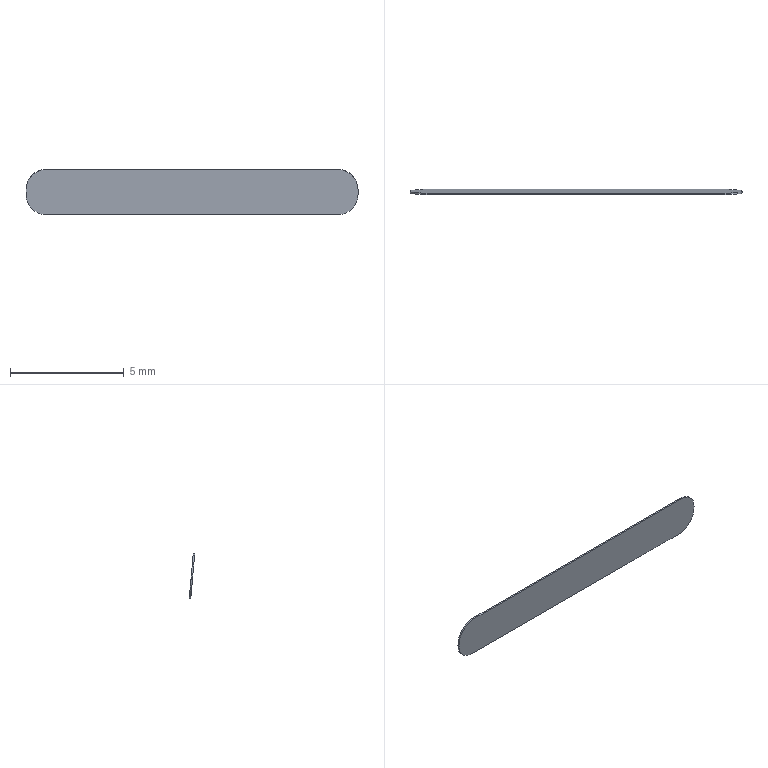Part | STEP file | p9-frame-03 | 1 solid | 10 faces | box 14.62 x 0.2371 x 1.998 mm | volume 1.798 mm3 | plane 6 | cylinder 4 | commonest cylinder face diameters 1.8 x4
STEP:
#1=CARTESIAN_POINT('',(27.35,-75.24,0.03301));
#2=VERTEX_POINT('',#1);
#3=CARTESIAN_POINT('',(26.45,-75.318,0.9296));
#4=VERTEX_POINT('',#3);
#5=CARTESIAN_POINT('',(26.45,-75.24,0.03301));
#6=DIRECTION('',(0.,-0.9962,-0.08716));
#7=DIRECTION('',(0.,-0.08716,0.9962));
#8=AXIS2_PLACEMENT_3D('',#5,#6,#7);
#9=CIRCLE('',#8,0.9);
#10=EDGE_CURVE('',#2,#4,#9,.T.);
#11=ORIENTED_EDGE('',*,*,#10,.F.);
#12=CARTESIAN_POINT('',(27.35,-75.222,-0.1662));
#13=VERTEX_POINT('',#12);
#14=CARTESIAN_POINT('',(27.35,-75.294,0.6557));
#15=DIRECTION('',(0.,-0.08716,0.9962));
#16=VECTOR('',#15,1000.);
#17=LINE('',#14,#16);
#18=EDGE_CURVE('',#13,#2,#17,.T.);
#19=ORIENTED_EDGE('',*,*,#18,.F.);
#20=CARTESIAN_POINT('',(26.45,-75.144,-1.063));
#21=VERTEX_POINT('',#20);
#22=CARTESIAN_POINT('',(26.45,-75.222,-0.1662));
#23=DIRECTION('',(0.,-0.9962,-0.08716));
#24=DIRECTION('',(0.,-0.08716,0.9962));
#25=AXIS2_PLACEMENT_3D('',#22,#23,#24);
#26=CIRCLE('',#25,0.9);
#27=EDGE_CURVE('',#21,#13,#26,.T.);
#28=ORIENTED_EDGE('',*,*,#27,.F.);
#29=CARTESIAN_POINT('',(13.63,-75.144,-1.063));
#30=VERTEX_POINT('',#29);
#31=CARTESIAN_POINT('',(2.234,-75.144,-1.063));
#32=DIRECTION('',(1.,0.,0.));
#33=VECTOR('',#32,1000.);
#34=LINE('',#31,#33);
#35=EDGE_CURVE('',#30,#21,#34,.T.);
#36=ORIENTED_EDGE('',*,*,#35,.F.);
#37=CARTESIAN_POINT('',(12.73,-75.222,-0.1662));
#38=VERTEX_POINT('',#37);
#39=CARTESIAN_POINT('',(13.63,-75.222,-0.1662));
#40=DIRECTION('',(0.,-0.9962,-0.08716));
#41=DIRECTION('',(0.,-0.08716,0.9962));
#42=AXIS2_PLACEMENT_3D('',#39,#40,#41);
#43=CIRCLE('',#42,0.9);
#44=EDGE_CURVE('',#38,#30,#43,.T.);
#45=ORIENTED_EDGE('',*,*,#44,.F.);
#46=CARTESIAN_POINT('',(12.73,-75.24,0.03301));
#47=VERTEX_POINT('',#46);
#48=CARTESIAN_POINT('',(12.73,-75.294,0.6557));
#49=DIRECTION('',(0.,0.08716,-0.9962));
#50=VECTOR('',#49,1000.);
#51=LINE('',#48,#50);
#52=EDGE_CURVE('',#47,#38,#51,.T.);
#53=ORIENTED_EDGE('',*,*,#52,.F.);
#54=CARTESIAN_POINT('',(13.63,-75.318,0.9296));
#55=VERTEX_POINT('',#54);
#56=CARTESIAN_POINT('',(13.63,-75.24,0.03301));
#57=DIRECTION('',(0.,-0.9962,-0.08716));
#58=DIRECTION('',(0.,-0.08716,0.9962));
#59=AXIS2_PLACEMENT_3D('',#56,#57,#58);
#60=CIRCLE('',#59,0.9);
#61=EDGE_CURVE('',#55,#47,#60,.T.);
#62=ORIENTED_EDGE('',*,*,#61,.F.);
#63=CARTESIAN_POINT('',(2.234,-75.318,0.9296));
#64=DIRECTION('',(-1.,0.,0.));
#65=VECTOR('',#64,1000.);
#66=LINE('',#63,#65);
#67=EDGE_CURVE('',#4,#55,#66,.T.);
#68=ORIENTED_EDGE('',*,*,#67,.F.);
#69=EDGE_LOOP('',(#11,#19,#28,#36,#45,#53,#62,#68));
#70=FACE_OUTER_BOUND('',#69,.T.);
#71=CARTESIAN_POINT('',(2.234,-75.294,0.6557));
#72=DIRECTION('',(0.,-0.9962,-0.08716));
#73=DIRECTION('',(0.,0.08716,-0.9962));
#74=AXIS2_PLACEMENT_3D('',#71,#72,#73);
#75=PLANE('',#74);
#76=ADVANCED_FACE('',(#70),#75,.F.);
#77=CARTESIAN_POINT('',(26.45,-75.381,0.9241));
#78=VERTEX_POINT('',#77);
#79=CARTESIAN_POINT('',(26.45,-75.717,0.8947));
#80=DIRECTION('',(0.,-0.9962,-0.08716));
#81=VECTOR('',#80,1000.);
#82=LINE('',#79,#81);
#83=EDGE_CURVE('',#4,#78,#82,.T.);
#84=ORIENTED_EDGE('',*,*,#83,.F.);
#85=ORIENTED_EDGE('',*,*,#67,.T.);
#86=CARTESIAN_POINT('',(13.63,-75.381,0.9241));
#87=VERTEX_POINT('',#86);
#88=CARTESIAN_POINT('',(13.63,-75.717,0.8947));
#89=DIRECTION('',(0.,0.9962,0.08716));
#90=VECTOR('',#89,1000.);
#91=LINE('',#88,#90);
#92=EDGE_CURVE('',#87,#55,#91,.T.);
#93=ORIENTED_EDGE('',*,*,#92,.F.);
#94=CARTESIAN_POINT('',(-31.59,-75.381,0.9241));
#95=DIRECTION('',(-1.,0.,0.));
#96=VECTOR('',#95,1000.);
#97=LINE('',#94,#96);
#98=EDGE_CURVE('',#78,#87,#97,.T.);
#99=ORIENTED_EDGE('',*,*,#98,.F.);
#100=EDGE_LOOP('',(#84,#85,#93,#99));
#101=FACE_OUTER_BOUND('',#100,.T.);
#102=CARTESIAN_POINT('',(-31.59,-75.717,0.8947));
#103=DIRECTION('',(0.,0.08716,-0.9962));
#104=DIRECTION('',(0.,0.9962,0.08716));
#105=AXIS2_PLACEMENT_3D('',#102,#103,#104);
#106=PLANE('',#105);
#107=ADVANCED_FACE('',(#101),#106,.F.);
#108=CARTESIAN_POINT('',(27.35,-75.302,0.02752));
#109=VERTEX_POINT('',#108);
#110=CARTESIAN_POINT('',(27.35,-76.511,-0.07823));
#111=DIRECTION('',(0.,0.9962,0.08716));
#112=VECTOR('',#111,1000.);
#113=LINE('',#110,#112);
#114=EDGE_CURVE('',#109,#2,#113,.T.);
#115=ORIENTED_EDGE('',*,*,#114,.T.);
#116=ORIENTED_EDGE('',*,*,#10,.T.);
#117=ORIENTED_EDGE('',*,*,#83,.T.);
#118=CARTESIAN_POINT('',(26.45,-75.302,0.02752));
#119=DIRECTION('',(0.,0.9962,0.08716));
#120=DIRECTION('',(0.,-0.08716,0.9962));
#121=AXIS2_PLACEMENT_3D('',#118,#119,#120);
#122=CIRCLE('',#121,0.9);
#123=EDGE_CURVE('',#78,#109,#122,.T.);
#124=ORIENTED_EDGE('',*,*,#123,.T.);
#125=EDGE_LOOP('',(#115,#116,#117,#124));
#126=FACE_OUTER_BOUND('',#125,.T.);
#127=CARTESIAN_POINT('',(26.45,-76.511,-0.07823));
#128=DIRECTION('',(0.,0.9962,0.08716));
#129=DIRECTION('',(0.,-0.08716,0.9962));
#130=AXIS2_PLACEMENT_3D('',#127,#128,#129);
#131=CYLINDRICAL_SURFACE('',#130,0.9);
#132=ADVANCED_FACE('',(#126),#131,.T.);
#133=ORIENTED_EDGE('',*,*,#18,.T.);
#134=ORIENTED_EDGE('',*,*,#114,.F.);
#135=CARTESIAN_POINT('',(27.35,-75.285,-0.1717));
#136=VERTEX_POINT('',#135);
#137=CARTESIAN_POINT('',(27.35,-75.302,0.02752));
#138=DIRECTION('',(0.,0.08716,-0.9962));
#139=VECTOR('',#138,1000.);
#140=LINE('',#137,#139);
#141=EDGE_CURVE('',#109,#136,#140,.T.);
#142=ORIENTED_EDGE('',*,*,#141,.T.);
#143=CARTESIAN_POINT('',(27.35,-75.285,-0.1717));
#144=DIRECTION('',(0.,0.9962,0.08716));
#145=VECTOR('',#144,1000.);
#146=LINE('',#143,#145);
#147=EDGE_CURVE('',#136,#13,#146,.T.);
#148=ORIENTED_EDGE('',*,*,#147,.T.);
#149=EDGE_LOOP('',(#133,#134,#142,#148));
#150=FACE_OUTER_BOUND('',#149,.T.);
#151=CARTESIAN_POINT('',(27.35,-75.229,-1.07));
#152=DIRECTION('',(1.,0.,0.));
#153=DIRECTION('',(0.,1.,0.));
#154=AXIS2_PLACEMENT_3D('',#151,#152,#153);
#155=PLANE('',#154);
#156=ADVANCED_FACE('',(#150),#155,.T.);
#157=CARTESIAN_POINT('',(26.45,-75.207,-1.068));
#158=VERTEX_POINT('',#157);
#159=CARTESIAN_POINT('',(26.45,-76.433,-1.176));
#160=DIRECTION('',(0.,0.9962,0.08716));
#161=VECTOR('',#160,1000.);
#162=LINE('',#159,#161);
#163=EDGE_CURVE('',#158,#21,#162,.T.);
#164=ORIENTED_EDGE('',*,*,#163,.T.);
#165=ORIENTED_EDGE('',*,*,#27,.T.);
#166=ORIENTED_EDGE('',*,*,#147,.F.);
#167=CARTESIAN_POINT('',(26.45,-75.285,-0.1717));
#168=DIRECTION('',(0.,0.9962,0.08716));
#169=DIRECTION('',(0.,-0.08716,0.9962));
#170=AXIS2_PLACEMENT_3D('',#167,#168,#169);
#171=CIRCLE('',#170,0.9);
#172=EDGE_CURVE('',#136,#158,#171,.T.);
#173=ORIENTED_EDGE('',*,*,#172,.T.);
#174=EDGE_LOOP('',(#164,#165,#166,#173));
#175=FACE_OUTER_BOUND('',#174,.T.);
#176=CARTESIAN_POINT('',(26.45,-76.511,-0.279));
#177=DIRECTION('',(0.,0.9962,0.08716));
#178=DIRECTION('',(0.,-0.08716,0.9962));
#179=AXIS2_PLACEMENT_3D('',#176,#177,#178);
#180=CYLINDRICAL_SURFACE('',#179,0.9);
#181=ADVANCED_FACE('',(#175),#180,.T.);
#182=CARTESIAN_POINT('',(13.63,-75.207,-1.068));
#183=VERTEX_POINT('',#182);
#184=CARTESIAN_POINT('',(12.73,-75.207,-1.068));
#185=DIRECTION('',(-1.,0.,0.));
#186=VECTOR('',#185,1000.);
#187=LINE('',#184,#186);
#188=EDGE_CURVE('',#158,#183,#187,.T.);
#189=ORIENTED_EDGE('',*,*,#188,.T.);
#190=CARTESIAN_POINT('',(13.63,-75.229,-1.07));
#191=DIRECTION('',(0.,0.9962,0.08716));
#192=VECTOR('',#191,1000.);
#193=LINE('',#190,#192);
#194=EDGE_CURVE('',#183,#30,#193,.T.);
#195=ORIENTED_EDGE('',*,*,#194,.T.);
#196=ORIENTED_EDGE('',*,*,#35,.T.);
#197=ORIENTED_EDGE('',*,*,#163,.F.);
#198=EDGE_LOOP('',(#189,#195,#196,#197));
#199=FACE_OUTER_BOUND('',#198,.T.);
#200=CARTESIAN_POINT('',(12.73,-75.229,-1.07));
#201=DIRECTION('',(0.,0.08716,-0.9962));
#202=DIRECTION('',(0.,0.9962,0.08716));
#203=AXIS2_PLACEMENT_3D('',#200,#201,#202);
#204=PLANE('',#203);
#205=ADVANCED_FACE('',(#199),#204,.T.);
#206=CARTESIAN_POINT('',(12.73,-75.285,-0.1717));
#207=VERTEX_POINT('',#206);
#208=CARTESIAN_POINT('',(12.73,-76.511,-0.279));
#209=DIRECTION('',(0.,0.9962,0.08716));
#210=VECTOR('',#209,1000.);
#211=LINE('',#208,#210);
#212=EDGE_CURVE('',#207,#38,#211,.T.);
#213=ORIENTED_EDGE('',*,*,#212,.T.);
#214=ORIENTED_EDGE('',*,*,#44,.T.);
#215=ORIENTED_EDGE('',*,*,#194,.F.);
#216=CARTESIAN_POINT('',(13.63,-75.285,-0.1717));
#217=DIRECTION('',(0.,0.9962,0.08716));
#218=DIRECTION('',(0.,-0.08716,0.9962));
#219=AXIS2_PLACEMENT_3D('',#216,#217,#218);
#220=CIRCLE('',#219,0.9);
#221=EDGE_CURVE('',#183,#207,#220,.T.);
#222=ORIENTED_EDGE('',*,*,#221,.T.);
#223=EDGE_LOOP('',(#213,#214,#215,#222));
#224=FACE_OUTER_BOUND('',#223,.T.);
#225=CARTESIAN_POINT('',(13.63,-76.511,-0.279));
#226=DIRECTION('',(0.,0.9962,0.08716));
#227=DIRECTION('',(0.,-0.08716,0.9962));
#228=AXIS2_PLACEMENT_3D('',#225,#226,#227);
#229=CYLINDRICAL_SURFACE('',#228,0.9);
#230=ADVANCED_FACE('',(#224),#229,.T.);
#231=CARTESIAN_POINT('',(12.73,-75.302,0.02752));
#232=VERTEX_POINT('',#231);
#233=CARTESIAN_POINT('',(12.73,-75.285,-0.1717));
#234=DIRECTION('',(0.,-0.08716,0.9962));
#235=VECTOR('',#234,1000.);
#236=LINE('',#233,#235);
#237=EDGE_CURVE('',#207,#232,#236,.T.);
#238=ORIENTED_EDGE('',*,*,#237,.T.);
#239=CARTESIAN_POINT('',(12.73,-75.302,0.02752));
#240=DIRECTION('',(0.,0.9962,0.08716));
#241=VECTOR('',#240,1000.);
#242=LINE('',#239,#241);
#243=EDGE_CURVE('',#232,#47,#242,.T.);
#244=ORIENTED_EDGE('',*,*,#243,.T.);
#245=ORIENTED_EDGE('',*,*,#52,.T.);
#246=ORIENTED_EDGE('',*,*,#212,.F.);
#247=EDGE_LOOP('',(#238,#244,#245,#246));
#248=FACE_OUTER_BOUND('',#247,.T.);
#249=CARTESIAN_POINT('',(12.73,-75.403,0.9222));
#250=DIRECTION('',(-1.,0.,0.));
#251=DIRECTION('',(0.,-1.,0.));
#252=AXIS2_PLACEMENT_3D('',#249,#250,#251);
#253=PLANE('',#252);
#254=ADVANCED_FACE('',(#248),#253,.T.);
#255=ORIENTED_EDGE('',*,*,#92,.T.);
#256=ORIENTED_EDGE('',*,*,#61,.T.);
#257=ORIENTED_EDGE('',*,*,#243,.F.);
#258=CARTESIAN_POINT('',(13.63,-75.302,0.02752));
#259=DIRECTION('',(0.,0.9962,0.08716));
#260=DIRECTION('',(0.,-0.08716,0.9962));
#261=AXIS2_PLACEMENT_3D('',#258,#259,#260);
#262=CIRCLE('',#261,0.9);
#263=EDGE_CURVE('',#232,#87,#262,.T.);
#264=ORIENTED_EDGE('',*,*,#263,.T.);
#265=EDGE_LOOP('',(#255,#256,#257,#264));
#266=FACE_OUTER_BOUND('',#265,.T.);
#267=CARTESIAN_POINT('',(13.63,-76.511,-0.07823));
#268=DIRECTION('',(0.,0.9962,0.08716));
#269=DIRECTION('',(0.,-0.08716,0.9962));
#270=AXIS2_PLACEMENT_3D('',#267,#268,#269);
#271=CYLINDRICAL_SURFACE('',#270,0.9);
#272=ADVANCED_FACE('',(#266),#271,.T.);
#273=ORIENTED_EDGE('',*,*,#98,.T.);
#274=ORIENTED_EDGE('',*,*,#263,.F.);
#275=ORIENTED_EDGE('',*,*,#237,.F.);
#276=ORIENTED_EDGE('',*,*,#221,.F.);
#277=ORIENTED_EDGE('',*,*,#188,.F.);
#278=ORIENTED_EDGE('',*,*,#172,.F.);
#279=ORIENTED_EDGE('',*,*,#141,.F.);
#280=ORIENTED_EDGE('',*,*,#123,.F.);
#281=EDGE_LOOP('',(#273,#274,#275,#276,#277,#278,#279,#280));
#282=FACE_OUTER_BOUND('',#281,.T.);
#283=CARTESIAN_POINT('',(2.234,-75.357,0.6503));
#284=DIRECTION('',(0.,-0.9962,-0.08716));
#285=DIRECTION('',(0.,0.08716,-0.9962));
#286=AXIS2_PLACEMENT_3D('',#283,#284,#285);
#287=PLANE('',#286);
#288=ADVANCED_FACE('',(#282),#287,.T.);
#289=CLOSED_SHELL('',(#76,#107,#132,#156,#181,#205,#230,#254,#272,#288));
#290=MANIFOLD_SOLID_BREP('',#289);
#291=CARTESIAN_POINT('',(0.,0.,0.));
#292=DIRECTION('',(0.,0.,1.));
#293=DIRECTION('',(1.,0.,0.));
#294=AXIS2_PLACEMENT_3D('',#291,#292,#293);
#295=(LENGTH_UNIT()NAMED_UNIT(*)SI_UNIT(.MILLI.,.METRE.));
#296=UNCERTAINTY_MEASURE_WITH_UNIT(LENGTH_MEASURE(0.00001),#295,'','');
#297=(NAMED_UNIT(*)PLANE_ANGLE_UNIT()SI_UNIT($,.RADIAN.));
#298=(NAMED_UNIT(*)SI_UNIT($,.STERADIAN.)SOLID_ANGLE_UNIT());
#299=(GEOMETRIC_REPRESENTATION_CONTEXT(3)GLOBAL_UNCERTAINTY_ASSIGNED_CONTEXT((#296))GLOBAL_UNIT_ASSIGNED_CONTEXT((#295,#297,#298))REPRESENTATION_CONTEXT('',''));
#300=ADVANCED_BREP_SHAPE_REPRESENTATION('',(#290,#294),#299);